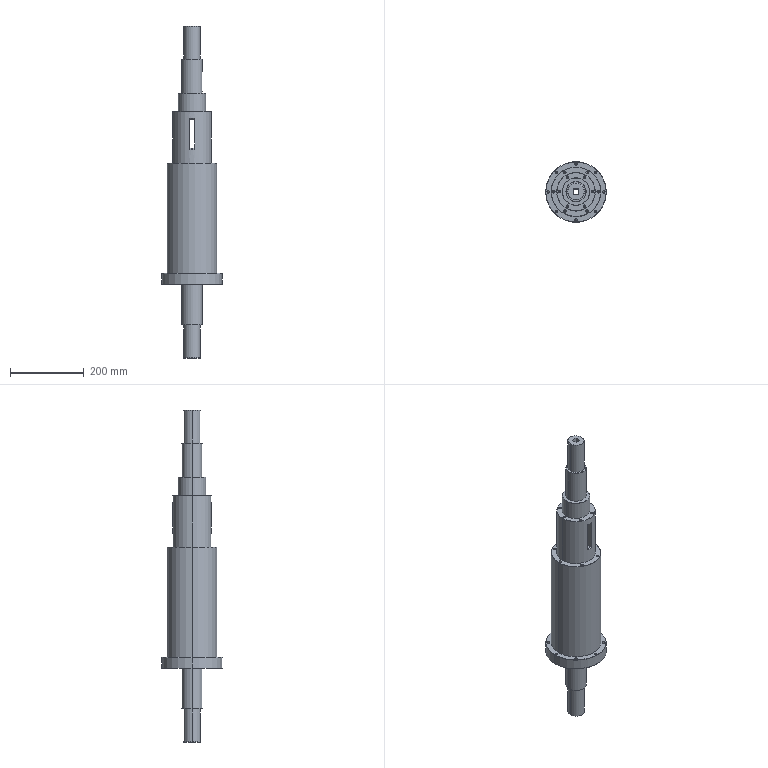Part | SolidWorks | features Chamfer 4, CirPattern 3, HoleWzd 3, ICE 2, Cut 1, Revolution 1 | 1 solid | 150 faces | box 165 x 165 x 903 mm | volume 6812270 mm3 | cone 62 | cylinder 58 | plane 30 | commonest cylinder face diameters 6.8 x40 45 x4 16 x2 55 x2 56 x2 75 x2